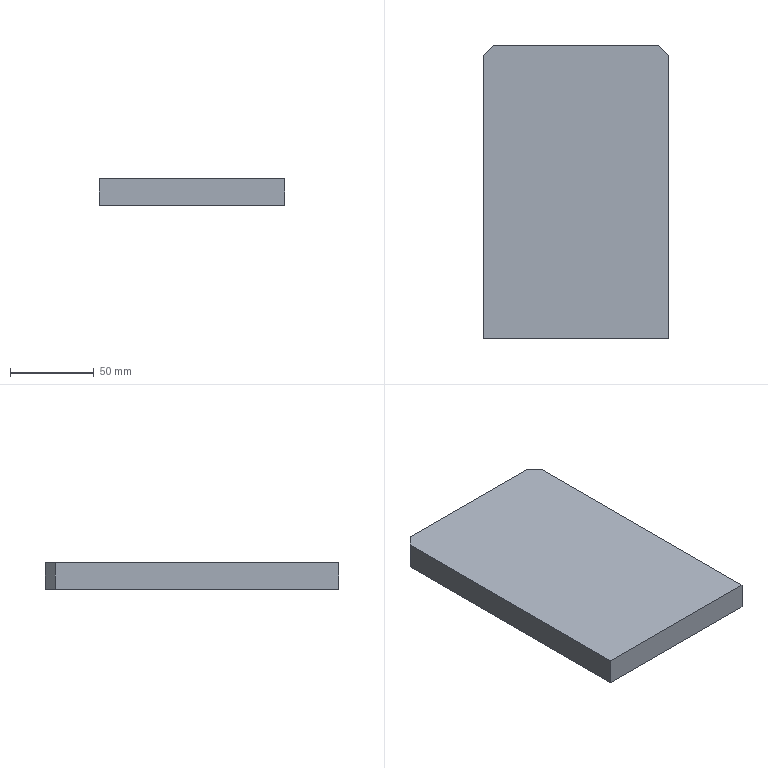Part | STEP file | ASND-0110-Rubbing imprint | 1 solid | 8 faces | box 111 x 175.7 x 16 mm | volume 311467 mm3 | plane 8
STEP:
#1=CARTESIAN_POINT('',(0.,0.,0.));
#2=DIRECTION('',(0.,0.,1.));
#3=DIRECTION('',(1.,0.,0.));
#4=AXIS2_PLACEMENT_3D('',#1,#2,#3);
#5=CARTESIAN_POINT('',(19.,141.7,16.));
#6=VERTEX_POINT('',#5);
#7=CARTESIAN_POINT('',(25.,147.7,16.));
#8=VERTEX_POINT('',#7);
#9=CARTESIAN_POINT('',(-15.175,107.525,16.));
#10=DIRECTION('',(0.7071,0.7071,0.));
#11=VECTOR('',#10,1.);
#12=LINE('',#9,#11);
#13=CARTESIAN_POINT('',(22.,144.7,16.));
#14=DIRECTION('',(-0.7071,0.7071,0.));
#15=DIRECTION('',(0.5774,0.5774,0.5774));
#16=AXIS2_PLACEMENT_3D('',#13,#14,#15);
#17=PLANE('',#16);
#18=CARTESIAN_POINT('',(-42.926,-30.353));
#19=DIRECTION('',(0.8165,0.5774));
#20=VECTOR('',#19,1.);
#21=LINE('',#18,#20);
#22=(GEOMETRIC_REPRESENTATION_CONTEXT(2)PARAMETRIC_REPRESENTATION_CONTEXT()REPRESENTATION_CONTEXT('',''));
#23=DEFINITIONAL_REPRESENTATION('',(#21),#22);
#24=PCURVE('',#17,#23);
#25=CARTESIAN_POINT('',(0.,0.,16.));
#26=DIRECTION('',(0.,0.,-1.));
#27=DIRECTION('',(0.7071,0.7071,0.));
#28=AXIS2_PLACEMENT_3D('',#25,#26,#27);
#29=PLANE('',#28);
#30=CARTESIAN_POINT('',(65.301,-86.762));
#31=DIRECTION('',(1.,0.));
#32=VECTOR('',#31,1.);
#33=LINE('',#30,#32);
#34=(GEOMETRIC_REPRESENTATION_CONTEXT(2)PARAMETRIC_REPRESENTATION_CONTEXT()REPRESENTATION_CONTEXT('',''));
#35=DEFINITIONAL_REPRESENTATION('',(#33),#34);
#36=PCURVE('',#29,#35);
#37=SURFACE_CURVE('',#12,(#24,#36),.PCURVE_S1.);
#38=EDGE_CURVE('',#6,#8,#37,.T.);
#39=ORIENTED_EDGE('',*,*,#38,.T.);
#40=CARTESIAN_POINT('',(25.,147.7,0.));
#41=VERTEX_POINT('',#40);
#42=CARTESIAN_POINT('',(25.,147.7,16.));
#43=DIRECTION('',(0.,0.,-1.));
#44=VECTOR('',#43,1.);
#45=LINE('',#42,#44);
#46=CARTESIAN_POINT('',(3.464,2.449));
#47=DIRECTION('',(-0.5774,0.8165));
#48=VECTOR('',#47,1.);
#49=LINE('',#46,#48);
#50=(GEOMETRIC_REPRESENTATION_CONTEXT(2)PARAMETRIC_REPRESENTATION_CONTEXT()REPRESENTATION_CONTEXT('',''));
#51=DEFINITIONAL_REPRESENTATION('',(#49),#50);
#52=PCURVE('',#17,#51);
#53=CARTESIAN_POINT('',(0.,147.7,16.));
#54=DIRECTION('',(0.,-1.,0.));
#55=DIRECTION('',(0.7071,0.,0.7071));
#56=AXIS2_PLACEMENT_3D('',#53,#54,#55);
#57=PLANE('',#56);
#58=CARTESIAN_POINT('',(17.678,-17.678));
#59=DIRECTION('',(-0.7071,-0.7071));
#60=VECTOR('',#59,1.);
#61=LINE('',#58,#60);
#62=(GEOMETRIC_REPRESENTATION_CONTEXT(2)PARAMETRIC_REPRESENTATION_CONTEXT()REPRESENTATION_CONTEXT('',''));
#63=DEFINITIONAL_REPRESENTATION('',(#61),#62);
#64=PCURVE('',#57,#63);
#65=SURFACE_CURVE('',#45,(#52,#64),.PCURVE_S1.);
#66=EDGE_CURVE('',#8,#41,#65,.T.);
#67=ORIENTED_EDGE('',*,*,#66,.T.);
#68=CARTESIAN_POINT('',(19.,141.7,0.));
#69=VERTEX_POINT('',#68);
#70=CARTESIAN_POINT('',(-15.175,107.525,0.));
#71=DIRECTION('',(-0.7071,-0.7071,0.));
#72=VECTOR('',#71,1.);
#73=LINE('',#70,#72);
#74=CARTESIAN_POINT('',(-52.164,-17.289));
#75=DIRECTION('',(-0.8165,-0.5774));
#76=VECTOR('',#75,1.);
#77=LINE('',#74,#76);
#78=(GEOMETRIC_REPRESENTATION_CONTEXT(2)PARAMETRIC_REPRESENTATION_CONTEXT()REPRESENTATION_CONTEXT('',''));
#79=DEFINITIONAL_REPRESENTATION('',(#77),#78);
#80=PCURVE('',#17,#79);
#81=CARTESIAN_POINT('',(0.,0.,0.));
#82=DIRECTION('',(0.,0.,-1.));
#83=DIRECTION('',(0.7071,0.7071,0.));
#84=AXIS2_PLACEMENT_3D('',#81,#82,#83);
#85=PLANE('',#84);
#86=CARTESIAN_POINT('',(65.301,-86.762));
#87=DIRECTION('',(-1.,0.));
#88=VECTOR('',#87,1.);
#89=LINE('',#86,#88);
#90=(GEOMETRIC_REPRESENTATION_CONTEXT(2)PARAMETRIC_REPRESENTATION_CONTEXT()REPRESENTATION_CONTEXT('',''));
#91=DEFINITIONAL_REPRESENTATION('',(#89),#90);
#92=PCURVE('',#85,#91);
#93=SURFACE_CURVE('',#73,(#80,#92),.PCURVE_S1.);
#94=EDGE_CURVE('',#41,#69,#93,.T.);
#95=ORIENTED_EDGE('',*,*,#94,.T.);
#96=CARTESIAN_POINT('',(19.,141.7,16.));
#97=DIRECTION('',(0.,0.,1.));
#98=VECTOR('',#97,1.);
#99=LINE('',#96,#98);
#100=CARTESIAN_POINT('',(-3.464,-2.449));
#101=DIRECTION('',(0.5774,-0.8165));
#102=VECTOR('',#101,1.);
#103=LINE('',#100,#102);
#104=(GEOMETRIC_REPRESENTATION_CONTEXT(2)PARAMETRIC_REPRESENTATION_CONTEXT()REPRESENTATION_CONTEXT('',''));
#105=DEFINITIONAL_REPRESENTATION('',(#103),#104);
#106=PCURVE('',#17,#105);
#107=CARTESIAN_POINT('',(19.,0.,16.));
#108=DIRECTION('',(1.,0.,0.));
#109=DIRECTION('',(0.,0.7071,0.7071));
#110=AXIS2_PLACEMENT_3D('',#107,#108,#109);
#111=PLANE('',#110);
#112=CARTESIAN_POINT('',(100.197,-100.197));
#113=DIRECTION('',(0.7071,0.7071));
#114=VECTOR('',#113,1.);
#115=LINE('',#112,#114);
#116=(GEOMETRIC_REPRESENTATION_CONTEXT(2)PARAMETRIC_REPRESENTATION_CONTEXT()REPRESENTATION_CONTEXT('',''));
#117=DEFINITIONAL_REPRESENTATION('',(#115),#116);
#118=PCURVE('',#111,#117);
#119=SURFACE_CURVE('',#99,(#106,#118),.PCURVE_S1.);
#120=EDGE_CURVE('',#69,#6,#119,.T.);
#121=ORIENTED_EDGE('',*,*,#120,.T.);
#122=EDGE_LOOP('',(#39,#67,#95,#121));
#123=FACE_BOUND('',#122,.T.);
#124=ADVANCED_FACE('',(#123),#17,.T.);
#125=ORIENTED_EDGE('',*,*,#66,.F.);
#126=CARTESIAN_POINT('',(124.,147.7,16.));
#127=VERTEX_POINT('',#126);
#128=CARTESIAN_POINT('',(140.,147.7,16.));
#129=DIRECTION('',(-1.,0.,0.));
#130=VECTOR('',#129,1.);
#131=LINE('',#128,#130);
#132=CARTESIAN_POINT('',(98.995,-98.995));
#133=DIRECTION('',(-0.7071,0.7071));
#134=VECTOR('',#133,1.);
#135=LINE('',#132,#134);
#136=(GEOMETRIC_REPRESENTATION_CONTEXT(2)PARAMETRIC_REPRESENTATION_CONTEXT()REPRESENTATION_CONTEXT('',''));
#137=DEFINITIONAL_REPRESENTATION('',(#135),#136);
#138=PCURVE('',#57,#137);
#139=CARTESIAN_POINT('',(203.435,-5.445));
#140=DIRECTION('',(-0.7071,-0.7071));
#141=VECTOR('',#140,1.);
#142=LINE('',#139,#141);
#143=(GEOMETRIC_REPRESENTATION_CONTEXT(2)PARAMETRIC_REPRESENTATION_CONTEXT()REPRESENTATION_CONTEXT('',''));
#144=DEFINITIONAL_REPRESENTATION('',(#142),#143);
#145=PCURVE('',#29,#144);
#146=SURFACE_CURVE('',#131,(#138,#145),.PCURVE_S1.);
#147=EDGE_CURVE('',#127,#8,#146,.T.);
#148=ORIENTED_EDGE('',*,*,#147,.F.);
#149=CARTESIAN_POINT('',(124.,147.7,0.));
#150=VERTEX_POINT('',#149);
#151=CARTESIAN_POINT('',(124.,147.7,16.));
#152=DIRECTION('',(0.,0.,1.));
#153=VECTOR('',#152,1.);
#154=LINE('',#151,#153);
#155=CARTESIAN_POINT('',(87.681,-87.681));
#156=DIRECTION('',(0.7071,0.7071));
#157=VECTOR('',#156,1.);
#158=LINE('',#155,#157);
#159=(GEOMETRIC_REPRESENTATION_CONTEXT(2)PARAMETRIC_REPRESENTATION_CONTEXT()REPRESENTATION_CONTEXT('',''));
#160=DEFINITIONAL_REPRESENTATION('',(#158),#159);
#161=PCURVE('',#57,#160);
#162=CARTESIAN_POINT('',(127.,144.7,16.));
#163=DIRECTION('',(0.7071,0.7071,0.));
#164=DIRECTION('',(-0.5774,0.5774,0.5774));
#165=AXIS2_PLACEMENT_3D('',#162,#163,#164);
#166=PLANE('',#165);
#167=CARTESIAN_POINT('',(3.464,-2.449));
#168=DIRECTION('',(0.5774,0.8165));
#169=VECTOR('',#168,1.);
#170=LINE('',#167,#169);
#171=(GEOMETRIC_REPRESENTATION_CONTEXT(2)PARAMETRIC_REPRESENTATION_CONTEXT()REPRESENTATION_CONTEXT('',''));
#172=DEFINITIONAL_REPRESENTATION('',(#170),#171);
#173=PCURVE('',#166,#172);
#174=SURFACE_CURVE('',#154,(#161,#173),.PCURVE_S1.);
#175=EDGE_CURVE('',#150,#127,#174,.T.);
#176=ORIENTED_EDGE('',*,*,#175,.F.);
#177=CARTESIAN_POINT('',(140.,147.7,0.));
#178=DIRECTION('',(-1.,0.,0.));
#179=VECTOR('',#178,1.);
#180=LINE('',#177,#179);
#181=CARTESIAN_POINT('',(87.681,-110.309));
#182=DIRECTION('',(-0.7071,0.7071));
#183=VECTOR('',#182,1.);
#184=LINE('',#181,#183);
#185=(GEOMETRIC_REPRESENTATION_CONTEXT(2)PARAMETRIC_REPRESENTATION_CONTEXT()REPRESENTATION_CONTEXT('',''));
#186=DEFINITIONAL_REPRESENTATION('',(#184),#185);
#187=PCURVE('',#57,#186);
#188=CARTESIAN_POINT('',(203.435,-5.445));
#189=DIRECTION('',(-0.7071,-0.7071));
#190=VECTOR('',#189,1.);
#191=LINE('',#188,#190);
#192=(GEOMETRIC_REPRESENTATION_CONTEXT(2)PARAMETRIC_REPRESENTATION_CONTEXT()REPRESENTATION_CONTEXT('',''));
#193=DEFINITIONAL_REPRESENTATION('',(#191),#192);
#194=PCURVE('',#85,#193);
#195=SURFACE_CURVE('',#180,(#187,#194),.PCURVE_S1.);
#196=EDGE_CURVE('',#150,#41,#195,.T.);
#197=ORIENTED_EDGE('',*,*,#196,.T.);
#198=EDGE_LOOP('',(#125,#148,#176,#197));
#199=FACE_BOUND('',#198,.T.);
#200=ADVANCED_FACE('',(#199),#57,.F.);
#201=ORIENTED_EDGE('',*,*,#38,.F.);
#202=CARTESIAN_POINT('',(19.,-28.,16.));
#203=VERTEX_POINT('',#202);
#204=CARTESIAN_POINT('',(19.,177.,16.));
#205=DIRECTION('',(0.,-1.,0.));
#206=VECTOR('',#205,1.);
#207=LINE('',#204,#206);
#208=CARTESIAN_POINT('',(138.593,-111.723));
#209=DIRECTION('',(-0.7071,0.7071));
#210=VECTOR('',#209,1.);
#211=LINE('',#208,#210);
#212=(GEOMETRIC_REPRESENTATION_CONTEXT(2)PARAMETRIC_REPRESENTATION_CONTEXT()REPRESENTATION_CONTEXT('',''));
#213=DEFINITIONAL_REPRESENTATION('',(#211),#212);
#214=PCURVE('',#29,#213);
#215=CARTESIAN_POINT('',(125.158,-125.158));
#216=DIRECTION('',(-0.7071,0.7071));
#217=VECTOR('',#216,1.);
#218=LINE('',#215,#217);
#219=(GEOMETRIC_REPRESENTATION_CONTEXT(2)PARAMETRIC_REPRESENTATION_CONTEXT()REPRESENTATION_CONTEXT('',''));
#220=DEFINITIONAL_REPRESENTATION('',(#218),#219);
#221=PCURVE('',#111,#220);
#222=SURFACE_CURVE('',#207,(#214,#221),.PCURVE_S1.);
#223=EDGE_CURVE('',#6,#203,#222,.T.);
#224=ORIENTED_EDGE('',*,*,#223,.T.);
#225=CARTESIAN_POINT('',(130.,-28.,16.));
#226=VERTEX_POINT('',#225);
#227=CARTESIAN_POINT('',(60.,-28.,16.));
#228=DIRECTION('',(1.,0.,0.));
#229=VECTOR('',#228,1.);
#230=LINE('',#227,#229);
#231=CARTESIAN_POINT('',(22.627,62.225));
#232=DIRECTION('',(0.7071,0.7071));
#233=VECTOR('',#232,1.);
#234=LINE('',#231,#233);
#235=(GEOMETRIC_REPRESENTATION_CONTEXT(2)PARAMETRIC_REPRESENTATION_CONTEXT()REPRESENTATION_CONTEXT('',''));
#236=DEFINITIONAL_REPRESENTATION('',(#234),#235);
#237=PCURVE('',#29,#236);
#238=CARTESIAN_POINT('',(0.,-28.,16.));
#239=DIRECTION('',(0.,1.,0.));
#240=DIRECTION('',(0.7071,0.,0.7071));
#241=AXIS2_PLACEMENT_3D('',#238,#239,#240);
#242=PLANE('',#241);
#243=CARTESIAN_POINT('',(42.426,42.426));
#244=DIRECTION('',(0.7071,0.7071));
#245=VECTOR('',#244,1.);
#246=LINE('',#243,#245);
#247=(GEOMETRIC_REPRESENTATION_CONTEXT(2)PARAMETRIC_REPRESENTATION_CONTEXT()REPRESENTATION_CONTEXT('',''));
#248=DEFINITIONAL_REPRESENTATION('',(#246),#247);
#249=PCURVE('',#242,#248);
#250=SURFACE_CURVE('',#230,(#237,#249),.PCURVE_S1.);
#251=EDGE_CURVE('',#203,#226,#250,.T.);
#252=ORIENTED_EDGE('',*,*,#251,.T.);
#253=CARTESIAN_POINT('',(130.,141.7,16.));
#254=VERTEX_POINT('',#253);
#255=CARTESIAN_POINT('',(130.,10.,16.));
#256=DIRECTION('',(0.,1.,0.));
#257=VECTOR('',#256,1.);
#258=LINE('',#255,#257);
#259=CARTESIAN_POINT('',(98.995,84.853));
#260=DIRECTION('',(0.7071,-0.7071));
#261=VECTOR('',#260,1.);
#262=LINE('',#259,#261);
#263=(GEOMETRIC_REPRESENTATION_CONTEXT(2)PARAMETRIC_REPRESENTATION_CONTEXT()REPRESENTATION_CONTEXT('',''));
#264=DEFINITIONAL_REPRESENTATION('',(#262),#263);
#265=PCURVE('',#29,#264);
#266=CARTESIAN_POINT('',(130.,0.,16.));
#267=DIRECTION('',(-1.,0.,0.));
#268=DIRECTION('',(0.,0.7071,0.7071));
#269=AXIS2_PLACEMENT_3D('',#266,#267,#268);
#270=PLANE('',#269);
#271=CARTESIAN_POINT('',(7.071,7.071));
#272=DIRECTION('',(0.7071,0.7071));
#273=VECTOR('',#272,1.);
#274=LINE('',#271,#273);
#275=(GEOMETRIC_REPRESENTATION_CONTEXT(2)PARAMETRIC_REPRESENTATION_CONTEXT()REPRESENTATION_CONTEXT('',''));
#276=DEFINITIONAL_REPRESENTATION('',(#274),#275);
#277=PCURVE('',#270,#276);
#278=SURFACE_CURVE('',#258,(#265,#277),.PCURVE_S1.);
#279=EDGE_CURVE('',#226,#254,#278,.T.);
#280=ORIENTED_EDGE('',*,*,#279,.T.);
#281=CARTESIAN_POINT('',(126.925,144.775,16.));
#282=DIRECTION('',(0.7071,-0.7071,0.));
#283=VECTOR('',#282,1.);
#284=LINE('',#281,#283);
#285=CARTESIAN_POINT('',(192.121,-12.622));
#286=DIRECTION('',(0.,1.));
#287=VECTOR('',#286,1.);
#288=LINE('',#285,#287);
#289=(GEOMETRIC_REPRESENTATION_CONTEXT(2)PARAMETRIC_REPRESENTATION_CONTEXT()REPRESENTATION_CONTEXT('',''));
#290=DEFINITIONAL_REPRESENTATION('',(#288),#289);
#291=PCURVE('',#29,#290);
#292=CARTESIAN_POINT('',(0.0866,-0.06124));
#293=DIRECTION('',(-0.8165,0.5774));
#294=VECTOR('',#293,1.);
#295=LINE('',#292,#294);
#296=(GEOMETRIC_REPRESENTATION_CONTEXT(2)PARAMETRIC_REPRESENTATION_CONTEXT()REPRESENTATION_CONTEXT('',''));
#297=DEFINITIONAL_REPRESENTATION('',(#295),#296);
#298=PCURVE('',#166,#297);
#299=SURFACE_CURVE('',#284,(#291,#298),.PCURVE_S1.);
#300=EDGE_CURVE('',#127,#254,#299,.T.);
#301=ORIENTED_EDGE('',*,*,#300,.F.);
#302=ORIENTED_EDGE('',*,*,#147,.T.);
#303=EDGE_LOOP('',(#201,#224,#252,#280,#301,#302));
#304=FACE_BOUND('',#303,.T.);
#305=ADVANCED_FACE('',(#304),#29,.F.);
#306=ORIENTED_EDGE('',*,*,#300,.T.);
#307=CARTESIAN_POINT('',(130.,141.7,0.));
#308=VERTEX_POINT('',#307);
#309=CARTESIAN_POINT('',(130.,141.7,16.));
#310=DIRECTION('',(0.,0.,-1.));
#311=VECTOR('',#310,1.);
#312=LINE('',#309,#311);
#313=CARTESIAN_POINT('',(-3.464,2.449));
#314=DIRECTION('',(-0.5774,-0.8165));
#315=VECTOR('',#314,1.);
#316=LINE('',#313,#315);
#317=(GEOMETRIC_REPRESENTATION_CONTEXT(2)PARAMETRIC_REPRESENTATION_CONTEXT()REPRESENTATION_CONTEXT('',''));
#318=DEFINITIONAL_REPRESENTATION('',(#316),#317);
#319=PCURVE('',#166,#318);
#320=CARTESIAN_POINT('',(100.197,100.197));
#321=DIRECTION('',(-0.7071,0.7071));
#322=VECTOR('',#321,1.);
#323=LINE('',#320,#322);
#324=(GEOMETRIC_REPRESENTATION_CONTEXT(2)PARAMETRIC_REPRESENTATION_CONTEXT()REPRESENTATION_CONTEXT('',''));
#325=DEFINITIONAL_REPRESENTATION('',(#323),#324);
#326=PCURVE('',#270,#325);
#327=SURFACE_CURVE('',#312,(#319,#326),.PCURVE_S1.);
#328=EDGE_CURVE('',#254,#308,#327,.T.);
#329=ORIENTED_EDGE('',*,*,#328,.T.);
#330=CARTESIAN_POINT('',(126.925,144.775,0.));
#331=DIRECTION('',(-0.7071,0.7071,0.));
#332=VECTOR('',#331,1.);
#333=LINE('',#330,#332);
#334=CARTESIAN_POINT('',(-9.151,-13.125));
#335=DIRECTION('',(0.8165,-0.5774));
#336=VECTOR('',#335,1.);
#337=LINE('',#334,#336);
#338=(GEOMETRIC_REPRESENTATION_CONTEXT(2)PARAMETRIC_REPRESENTATION_CONTEXT()REPRESENTATION_CONTEXT('',''));
#339=DEFINITIONAL_REPRESENTATION('',(#337),#338);
#340=PCURVE('',#166,#339);
#341=CARTESIAN_POINT('',(192.121,-12.622));
#342=DIRECTION('',(0.,-1.));
#343=VECTOR('',#342,1.);
#344=LINE('',#341,#343);
#345=(GEOMETRIC_REPRESENTATION_CONTEXT(2)PARAMETRIC_REPRESENTATION_CONTEXT()REPRESENTATION_CONTEXT('',''));
#346=DEFINITIONAL_REPRESENTATION('',(#344),#345);
#347=PCURVE('',#85,#346);
#348=SURFACE_CURVE('',#333,(#340,#347),.PCURVE_S1.);
#349=EDGE_CURVE('',#308,#150,#348,.T.);
#350=ORIENTED_EDGE('',*,*,#349,.T.);
#351=ORIENTED_EDGE('',*,*,#175,.T.);
#352=EDGE_LOOP('',(#306,#329,#350,#351));
#353=FACE_BOUND('',#352,.T.);
#354=ADVANCED_FACE('',(#353),#166,.T.);
#355=ORIENTED_EDGE('',*,*,#120,.F.);
#356=CARTESIAN_POINT('',(19.,-28.,0.));
#357=VERTEX_POINT('',#356);
#358=CARTESIAN_POINT('',(19.,177.,0.));
#359=DIRECTION('',(0.,-1.,0.));
#360=VECTOR('',#359,1.);
#361=LINE('',#358,#360);
#362=CARTESIAN_POINT('',(113.844,-136.472));
#363=DIRECTION('',(-0.7071,0.7071));
#364=VECTOR('',#363,1.);
#365=LINE('',#362,#364);
#366=(GEOMETRIC_REPRESENTATION_CONTEXT(2)PARAMETRIC_REPRESENTATION_CONTEXT()REPRESENTATION_CONTEXT('',''));
#367=DEFINITIONAL_REPRESENTATION('',(#365),#366);
#368=PCURVE('',#111,#367);
#369=CARTESIAN_POINT('',(138.593,-111.723));
#370=DIRECTION('',(-0.7071,0.7071));
#371=VECTOR('',#370,1.);
#372=LINE('',#369,#371);
#373=(GEOMETRIC_REPRESENTATION_CONTEXT(2)PARAMETRIC_REPRESENTATION_CONTEXT()REPRESENTATION_CONTEXT('',''));
#374=DEFINITIONAL_REPRESENTATION('',(#372),#373);
#375=PCURVE('',#85,#374);
#376=SURFACE_CURVE('',#361,(#368,#375),.PCURVE_S1.);
#377=EDGE_CURVE('',#69,#357,#376,.T.);
#378=ORIENTED_EDGE('',*,*,#377,.T.);
#379=CARTESIAN_POINT('',(19.,-28.,16.));
#380=DIRECTION('',(0.,0.,1.));
#381=VECTOR('',#380,1.);
#382=LINE('',#379,#381);
#383=CARTESIAN_POINT('',(-19.799,19.799));
#384=DIRECTION('',(0.7071,0.7071));
#385=VECTOR('',#384,1.);
#386=LINE('',#383,#385);
#387=(GEOMETRIC_REPRESENTATION_CONTEXT(2)PARAMETRIC_REPRESENTATION_CONTEXT()REPRESENTATION_CONTEXT('',''));
#388=DEFINITIONAL_REPRESENTATION('',(#386),#387);
#389=PCURVE('',#111,#388);
#390=CARTESIAN_POINT('',(13.435,13.435));
#391=DIRECTION('',(0.7071,-0.7071));
#392=VECTOR('',#391,1.);
#393=LINE('',#390,#392);
#394=(GEOMETRIC_REPRESENTATION_CONTEXT(2)PARAMETRIC_REPRESENTATION_CONTEXT()REPRESENTATION_CONTEXT('',''));
#395=DEFINITIONAL_REPRESENTATION('',(#393),#394);
#396=PCURVE('',#242,#395);
#397=SURFACE_CURVE('',#382,(#389,#396),.PCURVE_S1.);
#398=EDGE_CURVE('',#357,#203,#397,.T.);
#399=ORIENTED_EDGE('',*,*,#398,.T.);
#400=ORIENTED_EDGE('',*,*,#223,.F.);
#401=EDGE_LOOP('',(#355,#378,#399,#400));
#402=FACE_BOUND('',#401,.T.);
#403=ADVANCED_FACE('',(#402),#111,.F.);
#404=ORIENTED_EDGE('',*,*,#398,.F.);
#405=CARTESIAN_POINT('',(130.,-28.,0.));
#406=VERTEX_POINT('',#405);
#407=CARTESIAN_POINT('',(60.,-28.,0.));
#408=DIRECTION('',(1.,0.,0.));
#409=VECTOR('',#408,1.);
#410=LINE('',#407,#409);
#411=CARTESIAN_POINT('',(31.113,53.74));
#412=DIRECTION('',(0.7071,0.7071));
#413=VECTOR('',#412,1.);
#414=LINE('',#411,#413);
#415=(GEOMETRIC_REPRESENTATION_CONTEXT(2)PARAMETRIC_REPRESENTATION_CONTEXT()REPRESENTATION_CONTEXT('',''));
#416=DEFINITIONAL_REPRESENTATION('',(#414),#415);
#417=PCURVE('',#242,#416);
#418=CARTESIAN_POINT('',(22.627,62.225));
#419=DIRECTION('',(0.7071,0.7071));
#420=VECTOR('',#419,1.);
#421=LINE('',#418,#420);
#422=(GEOMETRIC_REPRESENTATION_CONTEXT(2)PARAMETRIC_REPRESENTATION_CONTEXT()REPRESENTATION_CONTEXT('',''));
#423=DEFINITIONAL_REPRESENTATION('',(#421),#422);
#424=PCURVE('',#85,#423);
#425=SURFACE_CURVE('',#410,(#417,#424),.PCURVE_S1.);
#426=EDGE_CURVE('',#357,#406,#425,.T.);
#427=ORIENTED_EDGE('',*,*,#426,.T.);
#428=CARTESIAN_POINT('',(130.,-28.,16.));
#429=DIRECTION('',(0.,0.,-1.));
#430=VECTOR('',#429,1.);
#431=LINE('',#428,#430);
#432=CARTESIAN_POINT('',(91.924,91.924));
#433=DIRECTION('',(-0.7071,0.7071));
#434=VECTOR('',#433,1.);
#435=LINE('',#432,#434);
#436=(GEOMETRIC_REPRESENTATION_CONTEXT(2)PARAMETRIC_REPRESENTATION_CONTEXT()REPRESENTATION_CONTEXT('',''));
#437=DEFINITIONAL_REPRESENTATION('',(#435),#436);
#438=PCURVE('',#242,#437);
#439=CARTESIAN_POINT('',(-19.799,-19.799));
#440=DIRECTION('',(-0.7071,0.7071));
#441=VECTOR('',#440,1.);
#442=LINE('',#439,#441);
#443=(GEOMETRIC_REPRESENTATION_CONTEXT(2)PARAMETRIC_REPRESENTATION_CONTEXT()REPRESENTATION_CONTEXT('',''));
#444=DEFINITIONAL_REPRESENTATION('',(#442),#443);
#445=PCURVE('',#270,#444);
#446=SURFACE_CURVE('',#431,(#438,#445),.PCURVE_S1.);
#447=EDGE_CURVE('',#226,#406,#446,.T.);
#448=ORIENTED_EDGE('',*,*,#447,.F.);
#449=ORIENTED_EDGE('',*,*,#251,.F.);
#450=EDGE_LOOP('',(#404,#427,#448,#449));
#451=FACE_BOUND('',#450,.T.);
#452=ADVANCED_FACE('',(#451),#242,.F.);
#453=ORIENTED_EDGE('',*,*,#94,.F.);
#454=ORIENTED_EDGE('',*,*,#196,.F.);
#455=ORIENTED_EDGE('',*,*,#349,.F.);
#456=CARTESIAN_POINT('',(130.,10.,0.));
#457=DIRECTION('',(0.,1.,0.));
#458=VECTOR('',#457,1.);
#459=LINE('',#456,#458);
#460=CARTESIAN_POINT('',(98.995,84.853));
#461=DIRECTION('',(0.7071,-0.7071));
#462=VECTOR('',#461,1.);
#463=LINE('',#460,#462);
#464=(GEOMETRIC_REPRESENTATION_CONTEXT(2)PARAMETRIC_REPRESENTATION_CONTEXT()REPRESENTATION_CONTEXT('',''));
#465=DEFINITIONAL_REPRESENTATION('',(#463),#464);
#466=PCURVE('',#85,#465);
#467=CARTESIAN_POINT('',(-4.243,18.385));
#468=DIRECTION('',(0.7071,0.7071));
#469=VECTOR('',#468,1.);
#470=LINE('',#467,#469);
#471=(GEOMETRIC_REPRESENTATION_CONTEXT(2)PARAMETRIC_REPRESENTATION_CONTEXT()REPRESENTATION_CONTEXT('',''));
#472=DEFINITIONAL_REPRESENTATION('',(#470),#471);
#473=PCURVE('',#270,#472);
#474=SURFACE_CURVE('',#459,(#466,#473),.PCURVE_S1.);
#475=EDGE_CURVE('',#406,#308,#474,.T.);
#476=ORIENTED_EDGE('',*,*,#475,.F.);
#477=ORIENTED_EDGE('',*,*,#426,.F.);
#478=ORIENTED_EDGE('',*,*,#377,.F.);
#479=EDGE_LOOP('',(#453,#454,#455,#476,#477,#478));
#480=FACE_BOUND('',#479,.T.);
#481=ADVANCED_FACE('',(#480),#85,.T.);
#482=ORIENTED_EDGE('',*,*,#328,.F.);
#483=ORIENTED_EDGE('',*,*,#279,.F.);
#484=ORIENTED_EDGE('',*,*,#447,.T.);
#485=ORIENTED_EDGE('',*,*,#475,.T.);
#486=EDGE_LOOP('',(#482,#483,#484,#485));
#487=FACE_BOUND('',#486,.T.);
#488=ADVANCED_FACE('',(#487),#270,.F.);
#489=CLOSED_SHELL('',(#124,#200,#305,#354,#403,#452,#481,#488));
#490=MANIFOLD_SOLID_BREP('',#489);
#491=(LENGTH_UNIT()NAMED_UNIT(*)SI_UNIT(.MILLI.,.METRE.));
#492=UNCERTAINTY_MEASURE_WITH_UNIT(LENGTH_MEASURE(0.0000001),#491,'','');
#493=(NAMED_UNIT(*)PLANE_ANGLE_UNIT()SI_UNIT($,.RADIAN.));
#494=(NAMED_UNIT(*)SI_UNIT($,.STERADIAN.)SOLID_ANGLE_UNIT());
#495=(GEOMETRIC_REPRESENTATION_CONTEXT(3)GLOBAL_UNCERTAINTY_ASSIGNED_CONTEXT((#492))GLOBAL_UNIT_ASSIGNED_CONTEXT((#491,#493,#494))REPRESENTATION_CONTEXT('',''));
#496=ADVANCED_BREP_SHAPE_REPRESENTATION('',(#4,#490),#495);